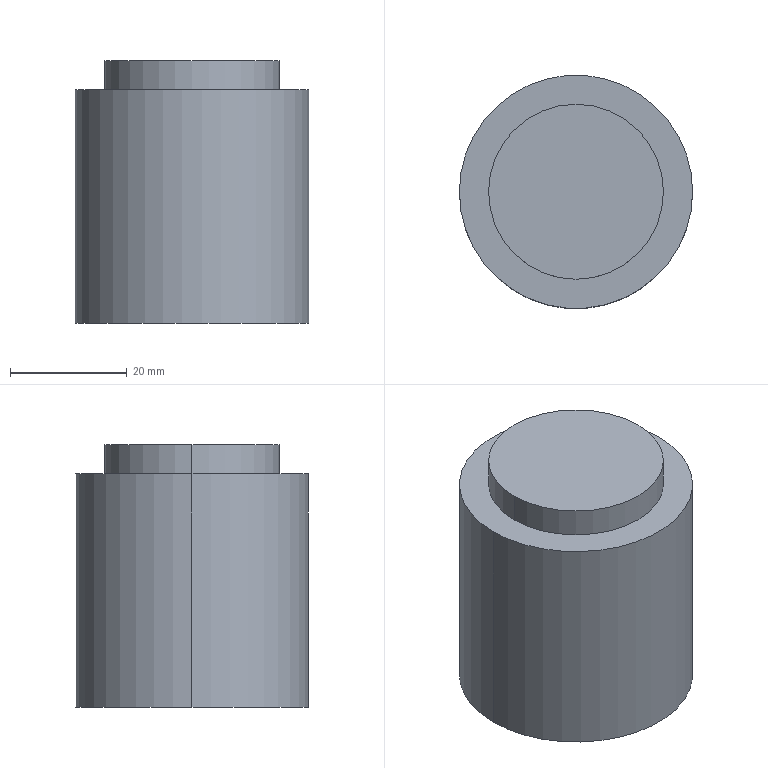Part | SolidWorks | features Extrusion 1, ICE 1 | 1 solid | 7 faces | box 40 x 40 x 45 mm | volume 53800 mm3 | cylinder 4 | plane 3 | commonest cylinder face diameters 30 x2 40 x2
STEP:
#1=CARTESIAN_POINT('',(15.,0.,45.));
#2=VERTEX_POINT('',#1);
#3=CARTESIAN_POINT('',(-15.,0.,45.));
#4=VERTEX_POINT('',#3);
#5=CARTESIAN_POINT('',(0.,0.,45.));
#6=DIRECTION('',(0.,0.,1.));
#7=DIRECTION('',(1.,0.,0.));
#8=AXIS2_PLACEMENT_3D('',#5,#6,#7);
#9=CIRCLE('',#8,15.);
#10=EDGE_CURVE('',#2,#4,#9,.T.);
#11=ORIENTED_EDGE('',*,*,#10,.F.);
#12=CARTESIAN_POINT('',(15.,0.,40.));
#13=VERTEX_POINT('',#12);
#14=CARTESIAN_POINT('',(15.,0.,45.));
#15=DIRECTION('',(0.,0.,-1.));
#16=VECTOR('',#15,1000.);
#17=LINE('',#14,#16);
#18=EDGE_CURVE('',#2,#13,#17,.T.);
#19=ORIENTED_EDGE('',*,*,#18,.T.);
#20=CARTESIAN_POINT('',(-15.,0.,40.));
#21=VERTEX_POINT('',#20);
#22=CARTESIAN_POINT('',(0.,0.,40.));
#23=DIRECTION('',(0.,0.,1.));
#24=DIRECTION('',(1.,0.,0.));
#25=AXIS2_PLACEMENT_3D('',#22,#23,#24);
#26=CIRCLE('',#25,15.);
#27=EDGE_CURVE('',#13,#21,#26,.T.);
#28=ORIENTED_EDGE('',*,*,#27,.T.);
#29=CARTESIAN_POINT('',(-15.,0.,45.));
#30=DIRECTION('',(0.,0.,-1.));
#31=VECTOR('',#30,1000.);
#32=LINE('',#29,#31);
#33=EDGE_CURVE('',#4,#21,#32,.T.);
#34=ORIENTED_EDGE('',*,*,#33,.F.);
#35=EDGE_LOOP('',(#11,#19,#28,#34));
#36=FACE_OUTER_BOUND('',#35,.T.);
#37=CARTESIAN_POINT('',(0.,0.,45.));
#38=DIRECTION('',(0.,0.,-1.));
#39=DIRECTION('',(-1.,0.,0.));
#40=AXIS2_PLACEMENT_3D('',#37,#38,#39);
#41=CYLINDRICAL_SURFACE('',#40,15.);
#42=ADVANCED_FACE('',(#36),#41,.T.);
#43=CARTESIAN_POINT('',(20.,0.,40.));
#44=VERTEX_POINT('',#43);
#45=CARTESIAN_POINT('',(-20.,0.,40.));
#46=VERTEX_POINT('',#45);
#47=CARTESIAN_POINT('',(0.,0.,40.));
#48=DIRECTION('',(0.,0.,1.));
#49=DIRECTION('',(1.,0.,0.));
#50=AXIS2_PLACEMENT_3D('',#47,#48,#49);
#51=CIRCLE('',#50,20.);
#52=EDGE_CURVE('',#44,#46,#51,.T.);
#53=ORIENTED_EDGE('',*,*,#52,.F.);
#54=CARTESIAN_POINT('',(20.,0.,0.));
#55=VERTEX_POINT('',#54);
#56=CARTESIAN_POINT('',(20.,0.,40.));
#57=DIRECTION('',(0.,0.,-1.));
#58=VECTOR('',#57,1000.);
#59=LINE('',#56,#58);
#60=EDGE_CURVE('',#44,#55,#59,.T.);
#61=ORIENTED_EDGE('',*,*,#60,.T.);
#62=CARTESIAN_POINT('',(-20.,0.,0.));
#63=VERTEX_POINT('',#62);
#64=CARTESIAN_POINT('',(0.,0.,0.));
#65=DIRECTION('',(0.,0.,1.));
#66=DIRECTION('',(1.,0.,0.));
#67=AXIS2_PLACEMENT_3D('',#64,#65,#66);
#68=CIRCLE('',#67,20.);
#69=EDGE_CURVE('',#55,#63,#68,.T.);
#70=ORIENTED_EDGE('',*,*,#69,.T.);
#71=CARTESIAN_POINT('',(-20.,0.,40.));
#72=DIRECTION('',(0.,0.,-1.));
#73=VECTOR('',#72,1000.);
#74=LINE('',#71,#73);
#75=EDGE_CURVE('',#46,#63,#74,.T.);
#76=ORIENTED_EDGE('',*,*,#75,.F.);
#77=EDGE_LOOP('',(#53,#61,#70,#76));
#78=FACE_OUTER_BOUND('',#77,.T.);
#79=CARTESIAN_POINT('',(0.,0.,40.));
#80=DIRECTION('',(0.,0.,-1.));
#81=DIRECTION('',(-1.,0.,0.));
#82=AXIS2_PLACEMENT_3D('',#79,#80,#81);
#83=CYLINDRICAL_SURFACE('',#82,20.);
#84=ADVANCED_FACE('',(#78),#83,.T.);
#85=ORIENTED_EDGE('',*,*,#60,.F.);
#86=CARTESIAN_POINT('',(0.,0.,40.));
#87=DIRECTION('',(0.,0.,1.));
#88=DIRECTION('',(1.,0.,0.));
#89=AXIS2_PLACEMENT_3D('',#86,#87,#88);
#90=CIRCLE('',#89,20.);
#91=EDGE_CURVE('',#46,#44,#90,.T.);
#92=ORIENTED_EDGE('',*,*,#91,.F.);
#93=ORIENTED_EDGE('',*,*,#75,.T.);
#94=CARTESIAN_POINT('',(0.,0.,0.));
#95=DIRECTION('',(0.,0.,1.));
#96=DIRECTION('',(1.,0.,0.));
#97=AXIS2_PLACEMENT_3D('',#94,#95,#96);
#98=CIRCLE('',#97,20.);
#99=EDGE_CURVE('',#63,#55,#98,.T.);
#100=ORIENTED_EDGE('',*,*,#99,.T.);
#101=EDGE_LOOP('',(#85,#92,#93,#100));
#102=FACE_OUTER_BOUND('',#101,.T.);
#103=CARTESIAN_POINT('',(0.,0.,40.));
#104=DIRECTION('',(0.,0.,-1.));
#105=DIRECTION('',(-1.,0.,0.));
#106=AXIS2_PLACEMENT_3D('',#103,#104,#105);
#107=CYLINDRICAL_SURFACE('',#106,20.);
#108=ADVANCED_FACE('',(#102),#107,.T.);
#109=CARTESIAN_POINT('',(0.,0.,40.));
#110=DIRECTION('',(0.,0.,1.));
#111=DIRECTION('',(1.,0.,0.));
#112=AXIS2_PLACEMENT_3D('',#109,#110,#111);
#113=CIRCLE('',#112,15.);
#114=EDGE_CURVE('',#21,#13,#113,.T.);
#115=ORIENTED_EDGE('',*,*,#114,.F.);
#116=ORIENTED_EDGE('',*,*,#27,.F.);
#117=EDGE_LOOP('',(#115,#116));
#118=FACE_BOUND('',#117,.T.);
#119=ORIENTED_EDGE('',*,*,#91,.T.);
#120=ORIENTED_EDGE('',*,*,#52,.T.);
#121=EDGE_LOOP('',(#119,#120));
#122=FACE_OUTER_BOUND('',#121,.T.);
#123=CARTESIAN_POINT('',(0.,0.,40.));
#124=DIRECTION('',(0.,0.,1.));
#125=DIRECTION('',(1.,0.,0.));
#126=AXIS2_PLACEMENT_3D('',#123,#124,#125);
#127=PLANE('',#126);
#128=ADVANCED_FACE('',(#118,#122),#127,.T.);
#129=ORIENTED_EDGE('',*,*,#99,.F.);
#130=ORIENTED_EDGE('',*,*,#69,.F.);
#131=EDGE_LOOP('',(#129,#130));
#132=FACE_OUTER_BOUND('',#131,.T.);
#133=CARTESIAN_POINT('',(0.,0.,0.));
#134=DIRECTION('',(0.,0.,1.));
#135=DIRECTION('',(1.,0.,0.));
#136=AXIS2_PLACEMENT_3D('',#133,#134,#135);
#137=PLANE('',#136);
#138=ADVANCED_FACE('',(#132),#137,.F.);
#139=ORIENTED_EDGE('',*,*,#18,.F.);
#140=CARTESIAN_POINT('',(0.,0.,45.));
#141=DIRECTION('',(0.,0.,1.));
#142=DIRECTION('',(1.,0.,0.));
#143=AXIS2_PLACEMENT_3D('',#140,#141,#142);
#144=CIRCLE('',#143,15.);
#145=EDGE_CURVE('',#4,#2,#144,.T.);
#146=ORIENTED_EDGE('',*,*,#145,.F.);
#147=ORIENTED_EDGE('',*,*,#33,.T.);
#148=ORIENTED_EDGE('',*,*,#114,.T.);
#149=EDGE_LOOP('',(#139,#146,#147,#148));
#150=FACE_OUTER_BOUND('',#149,.T.);
#151=CARTESIAN_POINT('',(0.,0.,45.));
#152=DIRECTION('',(0.,0.,-1.));
#153=DIRECTION('',(-1.,0.,0.));
#154=AXIS2_PLACEMENT_3D('',#151,#152,#153);
#155=CYLINDRICAL_SURFACE('',#154,15.);
#156=ADVANCED_FACE('',(#150),#155,.T.);
#157=ORIENTED_EDGE('',*,*,#145,.T.);
#158=ORIENTED_EDGE('',*,*,#10,.T.);
#159=EDGE_LOOP('',(#157,#158));
#160=FACE_OUTER_BOUND('',#159,.T.);
#161=CARTESIAN_POINT('',(0.,0.,45.));
#162=DIRECTION('',(0.,0.,1.));
#163=DIRECTION('',(1.,0.,0.));
#164=AXIS2_PLACEMENT_3D('',#161,#162,#163);
#165=PLANE('',#164);
#166=ADVANCED_FACE('',(#160),#165,.T.);
#167=CLOSED_SHELL('',(#42,#84,#108,#128,#138,#156,#166));
#168=MANIFOLD_SOLID_BREP('',#167);
#169=CARTESIAN_POINT('',(0.,0.,0.));
#170=DIRECTION('',(0.,0.,1.));
#171=DIRECTION('',(1.,0.,0.));
#172=AXIS2_PLACEMENT_3D('',#169,#170,#171);
#173=(LENGTH_UNIT()NAMED_UNIT(*)SI_UNIT(.MILLI.,.METRE.));
#174=UNCERTAINTY_MEASURE_WITH_UNIT(LENGTH_MEASURE(0.00001),#173,'','');
#175=(NAMED_UNIT(*)PLANE_ANGLE_UNIT()SI_UNIT($,.RADIAN.));
#176=(NAMED_UNIT(*)SI_UNIT($,.STERADIAN.)SOLID_ANGLE_UNIT());
#177=(GEOMETRIC_REPRESENTATION_CONTEXT(3)GLOBAL_UNCERTAINTY_ASSIGNED_CONTEXT((#174))GLOBAL_UNIT_ASSIGNED_CONTEXT((#173,#175,#176))REPRESENTATION_CONTEXT('',''));
#178=ADVANCED_BREP_SHAPE_REPRESENTATION('',(#168,#172),#177);